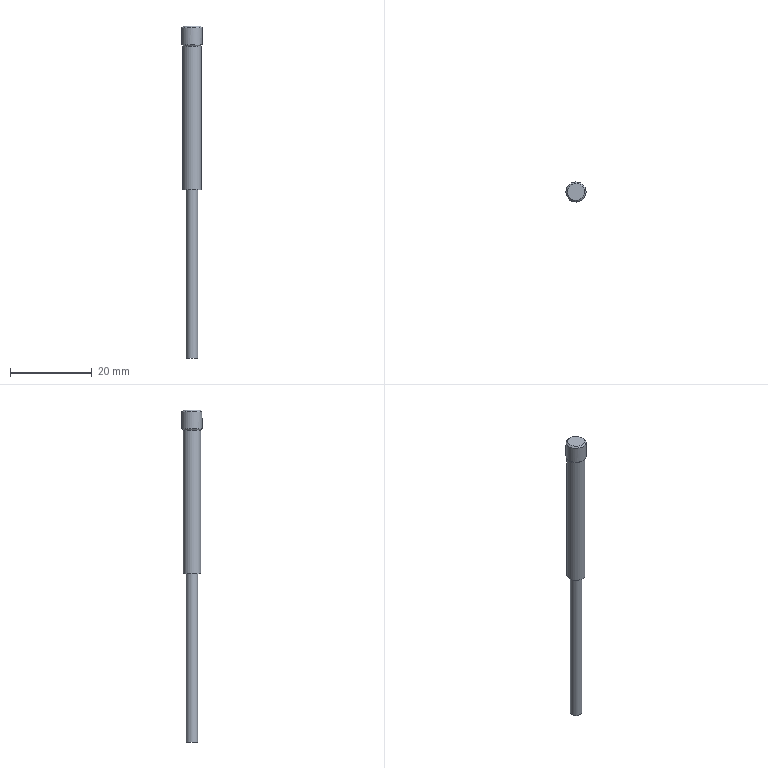Part | NX | features MI_APJAL_0250 2 | 1 solid | 9 faces | box 4.9 x 4.9 x 81 mm | volume 876.938 mm3 | cylinder 3 | plane 3 | spline 2 | cone 1 | commonest cylinder face diameters 2.8 x1 4.4 x1 4.9 x1
STEP:
#1=CARTESIAN_POINT('',(1283.879,141.904,35.1));
#2=VERTEX_POINT('',#1);
#3=CARTESIAN_POINT('',(1288.279,141.904,35.1));
#4=VERTEX_POINT('',#3);
#5=CARTESIAN_POINT('',(1286.079,141.904,35.1));
#6=DIRECTION('',(0.,0.,-1.));
#7=DIRECTION('',(1.,0.,0.));
#8=AXIS2_PLACEMENT_3D('',#5,#6,#7);
#9=CIRCLE('',#8,2.2);
#10=EDGE_CURVE('',#2,#4,#9,.T.);
#11=ORIENTED_EDGE('',*,*,#10,.F.);
#12=CARTESIAN_POINT('',(1283.629,141.904,35.448));
#13=VERTEX_POINT('',#12);
#14=CARTESIAN_POINT('',(1283.879,141.904,35.1));
#15=CARTESIAN_POINT('',(1283.796,141.904,35.216));
#16=CARTESIAN_POINT('',(1283.712,141.904,35.332));
#17=CARTESIAN_POINT('',(1283.629,141.904,35.449));
#18=B_SPLINE_CURVE_WITH_KNOTS('',3,(#14,#15,#16,#17),.UNSPECIFIED.,.F.,.F.,(4,4),(0.,1.),.UNSPECIFIED.);
#19=EDGE_CURVE('',#2,#13,#18,.T.);
#20=ORIENTED_EDGE('',*,*,#19,.T.);
#21=CARTESIAN_POINT('',(1286.057,144.354,35.448));
#22=VERTEX_POINT('',#21);
#23=CARTESIAN_POINT('',(1286.057,144.354,35.448));
#24=CARTESIAN_POINT('',(1285.759,144.351,35.448));
#25=CARTESIAN_POINT('',(1285.456,144.292,35.448));
#26=CARTESIAN_POINT('',(1284.885,144.066,35.448));
#27=CARTESIAN_POINT('',(1284.609,143.889,35.448));
#28=CARTESIAN_POINT('',(1284.153,143.451,35.448));
#29=CARTESIAN_POINT('',(1283.965,143.182,35.448));
#30=CARTESIAN_POINT('',(1283.71,142.604,35.448));
#31=CARTESIAN_POINT('',(1283.638,142.284,35.448));
#32=CARTESIAN_POINT('',(1283.629,141.947,35.448));
#33=CARTESIAN_POINT('',(1283.629,141.926,35.448));
#34=CARTESIAN_POINT('',(1283.629,141.904,35.448));
#35=B_SPLINE_CURVE_WITH_KNOTS('',3,(#23,#24,#25,#26,#27,#28,#29,#30,#31,#32,#33,#34),.UNSPECIFIED.,.F.,.F.,(4,2,2,2,2,4),(3.269,4.029,4.835,5.641,6.447,6.501),.UNSPECIFIED.);
#36=EDGE_CURVE('',#22,#13,#35,.T.);
#37=ORIENTED_EDGE('',*,*,#36,.F.);
#38=CARTESIAN_POINT('',(1288.529,141.904,35.448));
#39=VERTEX_POINT('',#38);
#40=CARTESIAN_POINT('',(1288.529,141.904,35.448));
#41=CARTESIAN_POINT('',(1288.529,142.22,35.448));
#42=CARTESIAN_POINT('',(1288.465,142.542,35.448));
#43=CARTESIAN_POINT('',(1288.225,143.127,35.448));
#44=CARTESIAN_POINT('',(1288.044,143.4,35.448));
#45=CARTESIAN_POINT('',(1287.601,143.85,35.448));
#46=CARTESIAN_POINT('',(1287.329,144.034,35.448));
#47=CARTESIAN_POINT('',(1286.748,144.282,35.448));
#48=CARTESIAN_POINT('',(1286.427,144.35,35.448));
#49=CARTESIAN_POINT('',(1286.093,144.354,35.448));
#50=CARTESIAN_POINT('',(1286.075,144.354,35.448));
#51=CARTESIAN_POINT('',(1286.057,144.354,35.448));
#52=B_SPLINE_CURVE_WITH_KNOTS('',3,(#40,#41,#42,#43,#44,#45,#46,#47,#48,#49,#50,#51),.UNSPECIFIED.,.F.,.F.,(4,2,2,2,2,4),(0.,0.8058,1.612,2.418,3.223,3.269),.UNSPECIFIED.);
#53=EDGE_CURVE('',#39,#22,#52,.T.);
#54=ORIENTED_EDGE('',*,*,#53,.F.);
#55=CARTESIAN_POINT('',(1288.529,141.902,35.448));
#56=VERTEX_POINT('',#55);
#57=CARTESIAN_POINT('',(1288.529,141.902,35.448));
#58=CARTESIAN_POINT('',(1288.529,141.903,35.448));
#59=CARTESIAN_POINT('',(1288.529,141.903,35.448));
#60=CARTESIAN_POINT('',(1288.529,141.904,35.448));
#61=B_SPLINE_CURVE_WITH_KNOTS('',3,(#57,#58,#59,#60),.UNSPECIFIED.,.F.,.F.,(4,4),(13.004,13.006),.UNSPECIFIED.);
#62=EDGE_CURVE('',#56,#39,#61,.T.);
#63=ORIENTED_EDGE('',*,*,#62,.F.);
#64=CARTESIAN_POINT('',(1288.279,141.902,35.1));
#65=VERTEX_POINT('',#64);
#66=CARTESIAN_POINT('',(1288.529,141.902,35.448));
#67=DIRECTION('',(-0.5832,0.0004724,-0.8123));
#68=VECTOR('',#67,1000.);
#69=LINE('',#66,#68);
#70=EDGE_CURVE('',#56,#65,#69,.T.);
#71=ORIENTED_EDGE('',*,*,#70,.T.);
#72=CARTESIAN_POINT('',(1286.079,141.904,35.1));
#73=DIRECTION('',(0.,0.,-1.));
#74=DIRECTION('',(1.,0.,0.));
#75=AXIS2_PLACEMENT_3D('',#72,#73,#74);
#76=CIRCLE('',#75,2.2);
#77=EDGE_CURVE('',#4,#65,#76,.T.);
#78=ORIENTED_EDGE('',*,*,#77,.F.);
#79=EDGE_LOOP('',(#11,#20,#37,#54,#63,#71,#78));
#80=FACE_BOUND('',#79,.T.);
#81=CARTESIAN_POINT('',(1283.879,141.904,35.1));
#82=CARTESIAN_POINT('',(1283.796,141.904,35.216));
#83=CARTESIAN_POINT('',(1283.712,141.904,35.332));
#84=CARTESIAN_POINT('',(1283.629,141.904,35.449));
#85=CARTESIAN_POINT('',(1283.879,142.066,35.1));
#86=CARTESIAN_POINT('',(1283.796,142.072,35.216));
#87=CARTESIAN_POINT('',(1283.713,142.078,35.332));
#88=CARTESIAN_POINT('',(1283.629,142.084,35.449));
#89=CARTESIAN_POINT('',(1283.897,142.228,35.1));
#90=CARTESIAN_POINT('',(1283.815,142.241,35.216));
#91=CARTESIAN_POINT('',(1283.732,142.253,35.332));
#92=CARTESIAN_POINT('',(1283.649,142.265,35.449));
#93=CARTESIAN_POINT('',(1283.968,142.544,35.1));
#94=CARTESIAN_POINT('',(1283.888,142.568,35.216));
#95=CARTESIAN_POINT('',(1283.808,142.592,35.332));
#96=CARTESIAN_POINT('',(1283.728,142.617,35.449));
#97=CARTESIAN_POINT('',(1284.021,142.699,35.1));
#98=CARTESIAN_POINT('',(1283.943,142.729,35.216));
#99=CARTESIAN_POINT('',(1283.866,142.759,35.332));
#100=CARTESIAN_POINT('',(1283.788,142.789,35.449));
#101=CARTESIAN_POINT('',(1284.212,143.101,35.1));
#102=CARTESIAN_POINT('',(1284.141,143.147,35.216));
#103=CARTESIAN_POINT('',(1284.071,143.192,35.332));
#104=CARTESIAN_POINT('',(1284.,143.238,35.449));
#105=CARTESIAN_POINT('',(1284.387,143.338,35.1));
#106=CARTESIAN_POINT('',(1284.323,143.393,35.216));
#107=CARTESIAN_POINT('',(1284.259,143.447,35.332));
#108=CARTESIAN_POINT('',(1284.195,143.501,35.449));
#109=CARTESIAN_POINT('',(1284.806,143.721,35.1));
#110=CARTESIAN_POINT('',(1284.758,143.789,35.216));
#111=CARTESIAN_POINT('',(1284.71,143.858,35.332));
#112=CARTESIAN_POINT('',(1284.662,143.927,35.448));
#113=CARTESIAN_POINT('',(1285.058,143.873,35.1));
#114=CARTESIAN_POINT('',(1285.02,143.948,35.216));
#115=CARTESIAN_POINT('',(1284.981,144.022,35.332));
#116=CARTESIAN_POINT('',(1284.942,144.097,35.448));
#117=CARTESIAN_POINT('',(1285.591,144.068,35.1));
#118=CARTESIAN_POINT('',(1285.573,144.15,35.216));
#119=CARTESIAN_POINT('',(1285.554,144.232,35.332));
#120=CARTESIAN_POINT('',(1285.536,144.314,35.448));
#121=CARTESIAN_POINT('',(1285.882,144.113,35.1));
#122=CARTESIAN_POINT('',(1285.875,144.197,35.216));
#123=CARTESIAN_POINT('',(1285.867,144.281,35.332));
#124=CARTESIAN_POINT('',(1285.86,144.364,35.448));
#125=CARTESIAN_POINT('',(1286.449,144.091,35.1));
#126=CARTESIAN_POINT('',(1286.464,144.174,35.216));
#127=CARTESIAN_POINT('',(1286.478,144.257,35.332));
#128=CARTESIAN_POINT('',(1286.492,144.339,35.448));
#129=CARTESIAN_POINT('',(1286.736,144.023,35.1));
#130=CARTESIAN_POINT('',(1286.761,144.103,35.216));
#131=CARTESIAN_POINT('',(1286.786,144.183,35.332));
#132=CARTESIAN_POINT('',(1286.811,144.263,35.448));
#133=CARTESIAN_POINT('',(1287.252,143.787,35.1));
#134=CARTESIAN_POINT('',(1287.297,143.858,35.216));
#135=CARTESIAN_POINT('',(1287.341,143.929,35.332));
#136=CARTESIAN_POINT('',(1287.385,144.001,35.448));
#137=CARTESIAN_POINT('',(1287.491,143.615,35.1));
#138=CARTESIAN_POINT('',(1287.545,143.679,35.216));
#139=CARTESIAN_POINT('',(1287.598,143.744,35.332));
#140=CARTESIAN_POINT('',(1287.652,143.809,35.448));
#141=CARTESIAN_POINT('',(1287.879,143.2,35.1));
#142=CARTESIAN_POINT('',(1287.947,143.249,35.216));
#143=CARTESIAN_POINT('',(1288.015,143.299,35.332));
#144=CARTESIAN_POINT('',(1288.084,143.348,35.448));
#145=CARTESIAN_POINT('',(1288.035,142.95,35.1));
#146=CARTESIAN_POINT('',(1288.109,142.99,35.216));
#147=CARTESIAN_POINT('',(1288.183,143.03,35.332));
#148=CARTESIAN_POINT('',(1288.257,143.069,35.448));
#149=CARTESIAN_POINT('',(1288.236,142.42,35.1));
#150=CARTESIAN_POINT('',(1288.318,142.439,35.216));
#151=CARTESIAN_POINT('',(1288.4,142.459,35.332));
#152=CARTESIAN_POINT('',(1288.482,142.479,35.448));
#153=CARTESIAN_POINT('',(1288.286,142.13,35.1));
#154=CARTESIAN_POINT('',(1288.369,142.138,35.216));
#155=CARTESIAN_POINT('',(1288.453,142.147,35.332));
#156=CARTESIAN_POINT('',(1288.537,142.155,35.448));
#157=CARTESIAN_POINT('',(1288.271,141.562,35.1));
#158=CARTESIAN_POINT('',(1288.354,141.549,35.216));
#159=CARTESIAN_POINT('',(1288.437,141.536,35.332));
#160=CARTESIAN_POINT('',(1288.52,141.523,35.448));
#161=CARTESIAN_POINT('',(1288.206,141.275,35.1));
#162=CARTESIAN_POINT('',(1288.287,141.251,35.216));
#163=CARTESIAN_POINT('',(1288.367,141.227,35.332));
#164=CARTESIAN_POINT('',(1288.448,141.203,35.448));
#165=CARTESIAN_POINT('',(1287.977,140.756,35.1));
#166=CARTESIAN_POINT('',(1288.049,140.712,35.216));
#167=CARTESIAN_POINT('',(1288.121,140.669,35.332));
#168=CARTESIAN_POINT('',(1288.193,140.625,35.448));
#169=CARTESIAN_POINT('',(1287.808,140.514,35.1));
#170=CARTESIAN_POINT('',(1287.874,140.462,35.216));
#171=CARTESIAN_POINT('',(1287.939,140.409,35.332));
#172=CARTESIAN_POINT('',(1288.005,140.357,35.448));
#173=CARTESIAN_POINT('',(1287.399,140.121,35.1));
#174=CARTESIAN_POINT('',(1287.449,140.054,35.216));
#175=CARTESIAN_POINT('',(1287.499,139.986,35.332));
#176=CARTESIAN_POINT('',(1287.549,139.919,35.448));
#177=CARTESIAN_POINT('',(1287.151,139.962,35.1));
#178=CARTESIAN_POINT('',(1287.192,139.888,35.216));
#179=CARTESIAN_POINT('',(1287.233,139.815,35.332));
#180=CARTESIAN_POINT('',(1287.273,139.741,35.448));
#181=CARTESIAN_POINT('',(1286.623,139.753,35.1));
#182=CARTESIAN_POINT('',(1286.644,139.672,35.216));
#183=CARTESIAN_POINT('',(1286.665,139.591,35.332));
#184=CARTESIAN_POINT('',(1286.685,139.509,35.448));
#185=CARTESIAN_POINT('',(1286.334,139.7,35.1));
#186=CARTESIAN_POINT('',(1286.343,139.617,35.216));
#187=CARTESIAN_POINT('',(1286.353,139.533,35.332));
#188=CARTESIAN_POINT('',(1286.363,139.45,35.448));
#189=CARTESIAN_POINT('',(1285.766,139.708,35.1));
#190=CARTESIAN_POINT('',(1285.754,139.625,35.216));
#191=CARTESIAN_POINT('',(1285.743,139.541,35.332));
#192=CARTESIAN_POINT('',(1285.731,139.458,35.448));
#193=CARTESIAN_POINT('',(1285.478,139.769,35.1));
#194=CARTESIAN_POINT('',(1285.455,139.688,35.216));
#195=CARTESIAN_POINT('',(1285.433,139.607,35.332));
#196=CARTESIAN_POINT('',(1285.41,139.526,35.448));
#197=CARTESIAN_POINT('',(1284.956,139.991,35.1));
#198=CARTESIAN_POINT('',(1284.913,139.919,35.216));
#199=CARTESIAN_POINT('',(1284.871,139.846,35.332));
#200=CARTESIAN_POINT('',(1284.828,139.774,35.448));
#201=CARTESIAN_POINT('',(1284.712,140.157,35.1));
#202=CARTESIAN_POINT('',(1284.661,140.09,35.216));
#203=CARTESIAN_POINT('',(1284.609,140.024,35.332));
#204=CARTESIAN_POINT('',(1284.557,139.958,35.448));
#205=CARTESIAN_POINT('',(1284.314,140.561,35.1));
#206=CARTESIAN_POINT('',(1284.247,140.51,35.216));
#207=CARTESIAN_POINT('',(1284.18,140.459,35.332));
#208=CARTESIAN_POINT('',(1284.113,140.408,35.448));
#209=CARTESIAN_POINT('',(1284.151,140.806,35.1));
#210=CARTESIAN_POINT('',(1284.078,140.765,35.216));
#211=CARTESIAN_POINT('',(1284.005,140.723,35.332));
#212=CARTESIAN_POINT('',(1283.932,140.682,35.448));
#213=CARTESIAN_POINT('',(1283.936,141.331,35.1));
#214=CARTESIAN_POINT('',(1283.855,141.31,35.216));
#215=CARTESIAN_POINT('',(1283.774,141.288,35.332));
#216=CARTESIAN_POINT('',(1283.693,141.266,35.448));
#217=CARTESIAN_POINT('',(1283.879,141.62,35.1));
#218=CARTESIAN_POINT('',(1283.796,141.61,35.216));
#219=CARTESIAN_POINT('',(1283.712,141.599,35.332));
#220=CARTESIAN_POINT('',(1283.629,141.588,35.448));
#221=CARTESIAN_POINT('',(1283.879,141.904,35.1));
#222=CARTESIAN_POINT('',(1283.796,141.904,35.216));
#223=CARTESIAN_POINT('',(1283.712,141.904,35.332));
#224=CARTESIAN_POINT('',(1283.629,141.904,35.449));
#225=B_SPLINE_SURFACE_WITH_KNOTS('',3,3,((#81,#82,#83,#84),(#85,#86,#87,#88),(#89,#90,#91,#92),(#93,#94,#95,#96),(#97,#98,#99,#100),(#101,#102,#103,#104),(#105,#106,#107,#108),(#109,#110,#111,#112),(#113,#114,#115,#116),(#117,#118,#119,#120),(#121,#122,#123,#124),(#125,#126,#127,#128),(#129,#130,#131,#132),(#133,#134,#135,#136),(#137,#138,#139,#140),(#141,#142,#143,#144),(#145,#146,#147,#148),(#149,#150,#151,#152),(#153,#154,#155,#156),(#157,#158,#159,#160),(#161,#162,#163,#164),(#165,#166,#167,#168),(#169,#170,#171,#172),(#173,#174,#175,#176),(#177,#178,#179,#180),(#181,#182,#183,#184),(#185,#186,#187,#188),(#189,#190,#191,#192),(#193,#194,#195,#196),(#197,#198,#199,#200),(#201,#202,#203,#204),(#205,#206,#207,#208),(#209,#210,#211,#212),(#213,#214,#215,#216),(#217,#218,#219,#220),(#221,#222,#223,#224)),.RULED_SURF.,.T.,.F.,.F.,(4,2,2,2,2,2,2,2,2,2,2,2,2,2,2,2,2,4),(4,4),(-13.006,-12.547,-12.088,-11.282,-10.476,-9.67,-8.864,-8.058,-7.253,-6.447,-5.641,-4.835,-4.029,-3.223,-2.418,-1.612,-0.8058,0.),(0.,1.),.UNSPECIFIED.);
#226=ADVANCED_FACE('',(#80),#225,.F.);
#227=CARTESIAN_POINT('',(1288.529,141.918,39.633));
#228=VERTEX_POINT('',#227);
#229=CARTESIAN_POINT('',(1283.629,141.904,39.633));
#230=VERTEX_POINT('',#229);
#231=CARTESIAN_POINT('',(1286.079,141.904,39.633));
#232=DIRECTION('',(0.,0.,-1.));
#233=DIRECTION('',(-1.,0.,0.));
#234=AXIS2_PLACEMENT_3D('',#231,#232,#233);
#235=CIRCLE('',#234,2.45);
#236=EDGE_CURVE('',#228,#230,#235,.T.);
#237=ORIENTED_EDGE('',*,*,#236,.T.);
#238=CARTESIAN_POINT('',(1286.057,144.354,39.633));
#239=VERTEX_POINT('',#238);
#240=CARTESIAN_POINT('',(1286.079,141.904,39.633));
#241=DIRECTION('',(0.,0.,-1.));
#242=DIRECTION('',(-1.,0.,0.));
#243=AXIS2_PLACEMENT_3D('',#240,#241,#242);
#244=CIRCLE('',#243,2.45);
#245=EDGE_CURVE('',#230,#239,#244,.T.);
#246=ORIENTED_EDGE('',*,*,#245,.T.);
#247=CARTESIAN_POINT('',(1286.057,144.354,39.632));
#248=CARTESIAN_POINT('',(1286.057,144.354,35.448));
#249=B_SPLINE_CURVE_WITH_KNOTS('',1,(#247,#248),.UNSPECIFIED.,.F.,.F.,(2,2),(0.08333,0.9167),.UNSPECIFIED.);
#250=EDGE_CURVE('',#239,#22,#249,.T.);
#251=ORIENTED_EDGE('',*,*,#250,.T.);
#252=ORIENTED_EDGE('',*,*,#36,.T.);
#253=CARTESIAN_POINT('',(1283.629,141.904,35.448));
#254=CARTESIAN_POINT('',(1283.629,141.609,35.448));
#255=CARTESIAN_POINT('',(1283.684,141.309,35.448));
#256=CARTESIAN_POINT('',(1283.901,140.738,35.448));
#257=CARTESIAN_POINT('',(1284.074,140.46,35.448));
#258=CARTESIAN_POINT('',(1284.506,139.999,35.448));
#259=CARTESIAN_POINT('',(1284.773,139.807,35.448));
#260=CARTESIAN_POINT('',(1285.348,139.544,35.448));
#261=CARTESIAN_POINT('',(1285.667,139.468,35.448));
#262=CARTESIAN_POINT('',(1286.298,139.443,35.448));
#263=CARTESIAN_POINT('',(1286.622,139.494,35.448));
#264=CARTESIAN_POINT('',(1287.216,139.711,35.448));
#265=CARTESIAN_POINT('',(1287.496,139.881,35.448));
#266=CARTESIAN_POINT('',(1287.963,140.307,35.448));
#267=CARTESIAN_POINT('',(1288.158,140.571,35.448));
#268=CARTESIAN_POINT('',(1288.37,141.019,35.448));
#269=CARTESIAN_POINT('',(1288.43,141.191,35.448));
#270=CARTESIAN_POINT('',(1288.509,141.542,35.448));
#271=CARTESIAN_POINT('',(1288.529,141.723,35.448));
#272=CARTESIAN_POINT('',(1288.529,141.902,35.448));
#273=B_SPLINE_CURVE_WITH_KNOTS('',3,(#253,#254,#255,#256,#257,#258,#259,#260,#261,#262,#263,#264,#265,#266,#267,#268,#269,#270,#271,#272),.UNSPECIFIED.,.F.,.F.,(4,2,2,2,2,2,2,2,2,4),(6.501,7.253,8.058,8.864,9.67,10.476,11.282,12.088,12.547,13.004),.UNSPECIFIED.);
#274=EDGE_CURVE('',#13,#56,#273,.T.);
#275=ORIENTED_EDGE('',*,*,#274,.T.);
#276=ORIENTED_EDGE('',*,*,#62,.T.);
#277=ORIENTED_EDGE('',*,*,#53,.T.);
#278=ORIENTED_EDGE('',*,*,#250,.F.);
#279=CARTESIAN_POINT('',(1286.079,141.904,39.633));
#280=DIRECTION('',(0.,0.,-1.));
#281=DIRECTION('',(-1.,0.,0.));
#282=AXIS2_PLACEMENT_3D('',#279,#280,#281);
#283=CIRCLE('',#282,2.45);
#284=EDGE_CURVE('',#239,#228,#283,.T.);
#285=ORIENTED_EDGE('',*,*,#284,.T.);
#286=EDGE_LOOP('',(#237,#246,#251,#252,#275,#276,#277,#278,#285));
#287=FACE_BOUND('',#286,.T.);
#288=CARTESIAN_POINT('',(1286.079,141.904,37.55));
#289=DIRECTION('',(0.,0.,-1.));
#290=DIRECTION('',(-0.008727,1.,0.));
#291=AXIS2_PLACEMENT_3D('',#288,#289,#290);
#292=CYLINDRICAL_SURFACE('',#291,2.45);
#293=ADVANCED_FACE('',(#287),#292,.T.);
#294=CARTESIAN_POINT('',(1283.996,141.904,40.));
#295=VERTEX_POINT('',#294);
#296=CARTESIAN_POINT('',(1288.161,141.916,40.));
#297=VERTEX_POINT('',#296);
#298=CARTESIAN_POINT('',(1286.079,141.904,40.));
#299=DIRECTION('',(0.,0.,1.));
#300=DIRECTION('',(-1.,0.,0.));
#301=AXIS2_PLACEMENT_3D('',#298,#299,#300);
#302=CIRCLE('',#301,2.083);
#303=EDGE_CURVE('',#295,#297,#302,.T.);
#304=ORIENTED_EDGE('',*,*,#303,.F.);
#305=CARTESIAN_POINT('',(1286.079,141.904,40.));
#306=DIRECTION('',(0.,0.,1.));
#307=DIRECTION('',(-1.,0.,0.));
#308=AXIS2_PLACEMENT_3D('',#305,#306,#307);
#309=CIRCLE('',#308,2.083);
#310=EDGE_CURVE('',#297,#295,#309,.T.);
#311=ORIENTED_EDGE('',*,*,#310,.F.);
#312=CARTESIAN_POINT('',(1288.161,141.916,40.));
#313=CARTESIAN_POINT('',(1288.529,141.918,39.633));
#314=B_SPLINE_CURVE_WITH_KNOTS('',1,(#312,#313),.UNSPECIFIED.,.F.,.F.,(2,2),(0.601,0.7071),.UNSPECIFIED.);
#315=EDGE_CURVE('',#297,#228,#314,.T.);
#316=ORIENTED_EDGE('',*,*,#315,.T.);
#317=ORIENTED_EDGE('',*,*,#284,.F.);
#318=ORIENTED_EDGE('',*,*,#245,.F.);
#319=ORIENTED_EDGE('',*,*,#236,.F.);
#320=ORIENTED_EDGE('',*,*,#315,.F.);
#321=EDGE_LOOP('',(#304,#311,#316,#317,#318,#319,#320));
#322=FACE_BOUND('',#321,.T.);
#323=CARTESIAN_POINT('',(1286.079,141.904,38.618));
#324=DIRECTION('',(0.,0.,-1.));
#325=DIRECTION('',(1.,0.005818,0.));
#326=AXIS2_PLACEMENT_3D('',#323,#324,#325);
#327=CONICAL_SURFACE('',#326,3.465,0.7854);
#328=ADVANCED_FACE('',(#322),#327,.T.);
#329=ORIENTED_EDGE('',*,*,#310,.T.);
#330=ORIENTED_EDGE('',*,*,#303,.T.);
#331=EDGE_LOOP('',(#329,#330));
#332=FACE_BOUND('',#331,.T.);
#333=CARTESIAN_POINT('',(1283.372,146.232,40.));
#334=DIRECTION('',(0.,0.,1.));
#335=DIRECTION('',(1.,0.,0.));
#336=AXIS2_PLACEMENT_3D('',#333,#334,#335);
#337=PLANE('',#336);
#338=ADVANCED_FACE('',(#332),#337,.T.);
#339=CARTESIAN_POINT('',(1284.679,141.904,0.));
#340=VERTEX_POINT('',#339);
#341=CARTESIAN_POINT('',(1286.079,141.904,0.));
#342=DIRECTION('',(0.,0.,-1.));
#343=DIRECTION('',(-1.,0.,0.));
#344=AXIS2_PLACEMENT_3D('',#341,#342,#343);
#345=CIRCLE('',#344,1.4);
#346=EDGE_CURVE('',#340,#340,#345,.T.);
#347=ORIENTED_EDGE('',*,*,#346,.T.);
#348=CARTESIAN_POINT('',(1284.679,141.904,-41.));
#349=VERTEX_POINT('',#348);
#350=CARTESIAN_POINT('',(1284.679,141.904,0.000001564));
#351=CARTESIAN_POINT('',(1284.679,141.904,-41.));
#352=B_SPLINE_CURVE_WITH_KNOTS('',1,(#350,#351),.UNSPECIFIED.,.F.,.F.,(2,2),(0.08333,0.9167),.UNSPECIFIED.);
#353=EDGE_CURVE('',#340,#349,#352,.T.);
#354=ORIENTED_EDGE('',*,*,#353,.T.);
#355=CARTESIAN_POINT('',(1286.079,141.904,-41.));
#356=DIRECTION('',(0.,0.,1.));
#357=DIRECTION('',(-1.,0.,0.));
#358=AXIS2_PLACEMENT_3D('',#355,#356,#357);
#359=CIRCLE('',#358,1.4);
#360=EDGE_CURVE('',#349,#349,#359,.T.);
#361=ORIENTED_EDGE('',*,*,#360,.T.);
#362=ORIENTED_EDGE('',*,*,#353,.F.);
#363=EDGE_LOOP('',(#347,#354,#361,#362));
#364=FACE_BOUND('',#363,.T.);
#365=CARTESIAN_POINT('',(1286.079,141.904,-20.5));
#366=DIRECTION('',(0.,0.,-1.));
#367=DIRECTION('',(-1.,0.,0.));
#368=AXIS2_PLACEMENT_3D('',#365,#366,#367);
#369=CYLINDRICAL_SURFACE('',#368,1.4);
#370=ADVANCED_FACE('',(#364),#369,.T.);
#371=ORIENTED_EDGE('',*,*,#360,.F.);
#372=EDGE_LOOP('',(#371));
#373=FACE_BOUND('',#372,.T.);
#374=CARTESIAN_POINT('',(1289.299,144.814,-41.));
#375=DIRECTION('',(0.,0.,-1.));
#376=DIRECTION('',(-1.,0.,0.));
#377=AXIS2_PLACEMENT_3D('',#374,#375,#376);
#378=PLANE('',#377);
#379=ADVANCED_FACE('',(#373),#378,.T.);
#380=ORIENTED_EDGE('',*,*,#10,.T.);
#381=ORIENTED_EDGE('',*,*,#77,.T.);
#382=CARTESIAN_POINT('',(1286.079,141.904,35.1));
#383=DIRECTION('',(0.,0.,-1.));
#384=DIRECTION('',(1.,0.,0.));
#385=AXIS2_PLACEMENT_3D('',#382,#383,#384);
#386=CIRCLE('',#385,2.2);
#387=EDGE_CURVE('',#65,#2,#386,.T.);
#388=ORIENTED_EDGE('',*,*,#387,.T.);
#389=CARTESIAN_POINT('',(1283.879,141.904,0.));
#390=VERTEX_POINT('',#389);
#391=CARTESIAN_POINT('',(1283.879,141.904,35.1));
#392=CARTESIAN_POINT('',(1283.879,141.904,0.000000456));
#393=B_SPLINE_CURVE_WITH_KNOTS('',1,(#391,#392),.UNSPECIFIED.,.F.,.F.,(2,2),(0.08333,0.9167),.UNSPECIFIED.);
#394=EDGE_CURVE('',#2,#390,#393,.T.);
#395=ORIENTED_EDGE('',*,*,#394,.T.);
#396=CARTESIAN_POINT('',(1286.079,141.904,0.));
#397=DIRECTION('',(0.,0.,1.));
#398=DIRECTION('',(-1.,0.,0.));
#399=AXIS2_PLACEMENT_3D('',#396,#397,#398);
#400=CIRCLE('',#399,2.2);
#401=EDGE_CURVE('',#390,#390,#400,.T.);
#402=ORIENTED_EDGE('',*,*,#401,.T.);
#403=ORIENTED_EDGE('',*,*,#394,.F.);
#404=EDGE_LOOP('',(#380,#381,#388,#395,#402,#403));
#405=FACE_BOUND('',#404,.T.);
#406=CARTESIAN_POINT('',(1286.079,141.904,17.55));
#407=DIRECTION('',(0.,0.,-1.));
#408=DIRECTION('',(-1.,0.,0.));
#409=AXIS2_PLACEMENT_3D('',#406,#407,#408);
#410=CYLINDRICAL_SURFACE('',#409,2.2);
#411=ADVANCED_FACE('',(#405),#410,.T.);
#412=ORIENTED_EDGE('',*,*,#401,.F.);
#413=EDGE_LOOP('',(#412));
#414=FACE_BOUND('',#413,.T.);
#415=ORIENTED_EDGE('',*,*,#346,.F.);
#416=EDGE_LOOP('',(#415));
#417=FACE_BOUND('',#416,.T.);
#418=CARTESIAN_POINT('',(1291.139,146.477,0.));
#419=DIRECTION('',(0.,0.,-1.));
#420=DIRECTION('',(-1.,0.,0.));
#421=AXIS2_PLACEMENT_3D('',#418,#419,#420);
#422=PLANE('',#421);
#423=ADVANCED_FACE('',(#414,#417),#422,.T.);
#424=ORIENTED_EDGE('',*,*,#274,.F.);
#425=ORIENTED_EDGE('',*,*,#19,.F.);
#426=ORIENTED_EDGE('',*,*,#387,.F.);
#427=ORIENTED_EDGE('',*,*,#70,.F.);
#428=EDGE_LOOP('',(#424,#425,#426,#427));
#429=FACE_BOUND('',#428,.T.);
#430=CARTESIAN_POINT('',(1283.879,141.904,35.1));
#431=CARTESIAN_POINT('',(1283.796,141.904,35.216));
#432=CARTESIAN_POINT('',(1283.712,141.904,35.332));
#433=CARTESIAN_POINT('',(1283.629,141.904,35.449));
#434=CARTESIAN_POINT('',(1283.879,142.066,35.1));
#435=CARTESIAN_POINT('',(1283.796,142.072,35.216));
#436=CARTESIAN_POINT('',(1283.713,142.078,35.332));
#437=CARTESIAN_POINT('',(1283.629,142.084,35.449));
#438=CARTESIAN_POINT('',(1283.897,142.228,35.1));
#439=CARTESIAN_POINT('',(1283.815,142.241,35.216));
#440=CARTESIAN_POINT('',(1283.732,142.253,35.332));
#441=CARTESIAN_POINT('',(1283.649,142.265,35.449));
#442=CARTESIAN_POINT('',(1283.968,142.544,35.1));
#443=CARTESIAN_POINT('',(1283.888,142.568,35.216));
#444=CARTESIAN_POINT('',(1283.808,142.592,35.332));
#445=CARTESIAN_POINT('',(1283.728,142.617,35.449));
#446=CARTESIAN_POINT('',(1284.021,142.699,35.1));
#447=CARTESIAN_POINT('',(1283.943,142.729,35.216));
#448=CARTESIAN_POINT('',(1283.866,142.759,35.332));
#449=CARTESIAN_POINT('',(1283.788,142.789,35.449));
#450=CARTESIAN_POINT('',(1284.212,143.101,35.1));
#451=CARTESIAN_POINT('',(1284.141,143.147,35.216));
#452=CARTESIAN_POINT('',(1284.071,143.192,35.332));
#453=CARTESIAN_POINT('',(1284.,143.238,35.449));
#454=CARTESIAN_POINT('',(1284.387,143.338,35.1));
#455=CARTESIAN_POINT('',(1284.323,143.393,35.216));
#456=CARTESIAN_POINT('',(1284.259,143.447,35.332));
#457=CARTESIAN_POINT('',(1284.195,143.501,35.449));
#458=CARTESIAN_POINT('',(1284.806,143.721,35.1));
#459=CARTESIAN_POINT('',(1284.758,143.789,35.216));
#460=CARTESIAN_POINT('',(1284.71,143.858,35.332));
#461=CARTESIAN_POINT('',(1284.662,143.927,35.448));
#462=CARTESIAN_POINT('',(1285.058,143.873,35.1));
#463=CARTESIAN_POINT('',(1285.02,143.948,35.216));
#464=CARTESIAN_POINT('',(1284.981,144.022,35.332));
#465=CARTESIAN_POINT('',(1284.942,144.097,35.448));
#466=CARTESIAN_POINT('',(1285.591,144.068,35.1));
#467=CARTESIAN_POINT('',(1285.573,144.15,35.216));
#468=CARTESIAN_POINT('',(1285.554,144.232,35.332));
#469=CARTESIAN_POINT('',(1285.536,144.314,35.448));
#470=CARTESIAN_POINT('',(1285.882,144.113,35.1));
#471=CARTESIAN_POINT('',(1285.875,144.197,35.216));
#472=CARTESIAN_POINT('',(1285.867,144.281,35.332));
#473=CARTESIAN_POINT('',(1285.86,144.364,35.448));
#474=CARTESIAN_POINT('',(1286.449,144.091,35.1));
#475=CARTESIAN_POINT('',(1286.464,144.174,35.216));
#476=CARTESIAN_POINT('',(1286.478,144.257,35.332));
#477=CARTESIAN_POINT('',(1286.492,144.339,35.448));
#478=CARTESIAN_POINT('',(1286.736,144.023,35.1));
#479=CARTESIAN_POINT('',(1286.761,144.103,35.216));
#480=CARTESIAN_POINT('',(1286.786,144.183,35.332));
#481=CARTESIAN_POINT('',(1286.811,144.263,35.448));
#482=CARTESIAN_POINT('',(1287.252,143.787,35.1));
#483=CARTESIAN_POINT('',(1287.297,143.858,35.216));
#484=CARTESIAN_POINT('',(1287.341,143.929,35.332));
#485=CARTESIAN_POINT('',(1287.385,144.001,35.448));
#486=CARTESIAN_POINT('',(1287.491,143.615,35.1));
#487=CARTESIAN_POINT('',(1287.545,143.679,35.216));
#488=CARTESIAN_POINT('',(1287.598,143.744,35.332));
#489=CARTESIAN_POINT('',(1287.652,143.809,35.448));
#490=CARTESIAN_POINT('',(1287.879,143.2,35.1));
#491=CARTESIAN_POINT('',(1287.947,143.249,35.216));
#492=CARTESIAN_POINT('',(1288.015,143.299,35.332));
#493=CARTESIAN_POINT('',(1288.084,143.348,35.448));
#494=CARTESIAN_POINT('',(1288.035,142.95,35.1));
#495=CARTESIAN_POINT('',(1288.109,142.99,35.216));
#496=CARTESIAN_POINT('',(1288.183,143.03,35.332));
#497=CARTESIAN_POINT('',(1288.257,143.069,35.448));
#498=CARTESIAN_POINT('',(1288.236,142.42,35.1));
#499=CARTESIAN_POINT('',(1288.318,142.439,35.216));
#500=CARTESIAN_POINT('',(1288.4,142.459,35.332));
#501=CARTESIAN_POINT('',(1288.482,142.479,35.448));
#502=CARTESIAN_POINT('',(1288.286,142.13,35.1));
#503=CARTESIAN_POINT('',(1288.369,142.138,35.216));
#504=CARTESIAN_POINT('',(1288.453,142.147,35.332));
#505=CARTESIAN_POINT('',(1288.537,142.155,35.448));
#506=CARTESIAN_POINT('',(1288.271,141.562,35.1));
#507=CARTESIAN_POINT('',(1288.354,141.549,35.216));
#508=CARTESIAN_POINT('',(1288.437,141.536,35.332));
#509=CARTESIAN_POINT('',(1288.52,141.523,35.448));
#510=CARTESIAN_POINT('',(1288.206,141.275,35.1));
#511=CARTESIAN_POINT('',(1288.287,141.251,35.216));
#512=CARTESIAN_POINT('',(1288.367,141.227,35.332));
#513=CARTESIAN_POINT('',(1288.448,141.203,35.448));
#514=CARTESIAN_POINT('',(1287.977,140.756,35.1));
#515=CARTESIAN_POINT('',(1288.049,140.712,35.216));
#516=CARTESIAN_POINT('',(1288.121,140.669,35.332));
#517=CARTESIAN_POINT('',(1288.193,140.625,35.448));
#518=CARTESIAN_POINT('',(1287.808,140.514,35.1));
#519=CARTESIAN_POINT('',(1287.874,140.462,35.216));
#520=CARTESIAN_POINT('',(1287.939,140.409,35.332));
#521=CARTESIAN_POINT('',(1288.005,140.357,35.448));
#522=CARTESIAN_POINT('',(1287.399,140.121,35.1));
#523=CARTESIAN_POINT('',(1287.449,140.054,35.216));
#524=CARTESIAN_POINT('',(1287.499,139.986,35.332));
#525=CARTESIAN_POINT('',(1287.549,139.919,35.448));
#526=CARTESIAN_POINT('',(1287.151,139.962,35.1));
#527=CARTESIAN_POINT('',(1287.192,139.888,35.216));
#528=CARTESIAN_POINT('',(1287.233,139.815,35.332));
#529=CARTESIAN_POINT('',(1287.273,139.741,35.448));
#530=CARTESIAN_POINT('',(1286.623,139.753,35.1));
#531=CARTESIAN_POINT('',(1286.644,139.672,35.216));
#532=CARTESIAN_POINT('',(1286.665,139.591,35.332));
#533=CARTESIAN_POINT('',(1286.685,139.509,35.448));
#534=CARTESIAN_POINT('',(1286.334,139.7,35.1));
#535=CARTESIAN_POINT('',(1286.343,139.617,35.216));
#536=CARTESIAN_POINT('',(1286.353,139.533,35.332));
#537=CARTESIAN_POINT('',(1286.363,139.45,35.448));
#538=CARTESIAN_POINT('',(1285.766,139.708,35.1));
#539=CARTESIAN_POINT('',(1285.754,139.625,35.216));
#540=CARTESIAN_POINT('',(1285.743,139.541,35.332));
#541=CARTESIAN_POINT('',(1285.731,139.458,35.448));
#542=CARTESIAN_POINT('',(1285.478,139.769,35.1));
#543=CARTESIAN_POINT('',(1285.455,139.688,35.216));
#544=CARTESIAN_POINT('',(1285.433,139.607,35.332));
#545=CARTESIAN_POINT('',(1285.41,139.526,35.448));
#546=CARTESIAN_POINT('',(1284.956,139.991,35.1));
#547=CARTESIAN_POINT('',(1284.913,139.919,35.216));
#548=CARTESIAN_POINT('',(1284.871,139.846,35.332));
#549=CARTESIAN_POINT('',(1284.828,139.774,35.448));
#550=CARTESIAN_POINT('',(1284.712,140.157,35.1));
#551=CARTESIAN_POINT('',(1284.661,140.09,35.216));
#552=CARTESIAN_POINT('',(1284.609,140.024,35.332));
#553=CARTESIAN_POINT('',(1284.557,139.958,35.448));
#554=CARTESIAN_POINT('',(1284.314,140.561,35.1));
#555=CARTESIAN_POINT('',(1284.247,140.51,35.216));
#556=CARTESIAN_POINT('',(1284.18,140.459,35.332));
#557=CARTESIAN_POINT('',(1284.113,140.408,35.448));
#558=CARTESIAN_POINT('',(1284.151,140.806,35.1));
#559=CARTESIAN_POINT('',(1284.078,140.765,35.216));
#560=CARTESIAN_POINT('',(1284.005,140.723,35.332));
#561=CARTESIAN_POINT('',(1283.932,140.682,35.448));
#562=CARTESIAN_POINT('',(1283.936,141.331,35.1));
#563=CARTESIAN_POINT('',(1283.855,141.31,35.216));
#564=CARTESIAN_POINT('',(1283.774,141.288,35.332));
#565=CARTESIAN_POINT('',(1283.693,141.266,35.448));
#566=CARTESIAN_POINT('',(1283.879,141.62,35.1));
#567=CARTESIAN_POINT('',(1283.796,141.61,35.216));
#568=CARTESIAN_POINT('',(1283.712,141.599,35.332));
#569=CARTESIAN_POINT('',(1283.629,141.588,35.448));
#570=CARTESIAN_POINT('',(1283.879,141.904,35.1));
#571=CARTESIAN_POINT('',(1283.796,141.904,35.216));
#572=CARTESIAN_POINT('',(1283.712,141.904,35.332));
#573=CARTESIAN_POINT('',(1283.629,141.904,35.449));
#574=B_SPLINE_SURFACE_WITH_KNOTS('',3,3,((#430,#431,#432,#433),(#434,#435,#436,#437),(#438,#439,#440,#441),(#442,#443,#444,#445),(#446,#447,#448,#449),(#450,#451,#452,#453),(#454,#455,#456,#457),(#458,#459,#460,#461),(#462,#463,#464,#465),(#466,#467,#468,#469),(#470,#471,#472,#473),(#474,#475,#476,#477),(#478,#479,#480,#481),(#482,#483,#484,#485),(#486,#487,#488,#489),(#490,#491,#492,#493),(#494,#495,#496,#497),(#498,#499,#500,#501),(#502,#503,#504,#505),(#506,#507,#508,#509),(#510,#511,#512,#513),(#514,#515,#516,#517),(#518,#519,#520,#521),(#522,#523,#524,#525),(#526,#527,#528,#529),(#530,#531,#532,#533),(#534,#535,#536,#537),(#538,#539,#540,#541),(#542,#543,#544,#545),(#546,#547,#548,#549),(#550,#551,#552,#553),(#554,#555,#556,#557),(#558,#559,#560,#561),(#562,#563,#564,#565),(#566,#567,#568,#569),(#570,#571,#572,#573)),.RULED_SURF.,.T.,.F.,.F.,(4,2,2,2,2,2,2,2,2,2,2,2,2,2,2,2,2,4),(4,4),(-13.006,-12.547,-12.088,-11.282,-10.476,-9.67,-8.864,-8.058,-7.253,-6.447,-5.641,-4.835,-4.029,-3.223,-2.418,-1.612,-0.8058,0.),(0.,1.),.UNSPECIFIED.);
#575=ADVANCED_FACE('',(#429),#574,.F.);
#576=CLOSED_SHELL('',(#226,#293,#328,#338,#370,#379,#411,#423,#575));
#577=MANIFOLD_SOLID_BREP('',#576);
#578=(LENGTH_UNIT()NAMED_UNIT(*)SI_UNIT(.MILLI.,.METRE.));
#579=UNCERTAINTY_MEASURE_WITH_UNIT(LENGTH_MEASURE(0.00001),#578,'','');
#580=(NAMED_UNIT(*)PLANE_ANGLE_UNIT()SI_UNIT($,.RADIAN.));
#581=(NAMED_UNIT(*)SI_UNIT($,.STERADIAN.)SOLID_ANGLE_UNIT());
#582=(GEOMETRIC_REPRESENTATION_CONTEXT(3)GLOBAL_UNCERTAINTY_ASSIGNED_CONTEXT((#579))GLOBAL_UNIT_ASSIGNED_CONTEXT((#578,#580,#581))REPRESENTATION_CONTEXT('',''));
#583=ADVANCED_BREP_SHAPE_REPRESENTATION('',(#577),#582);